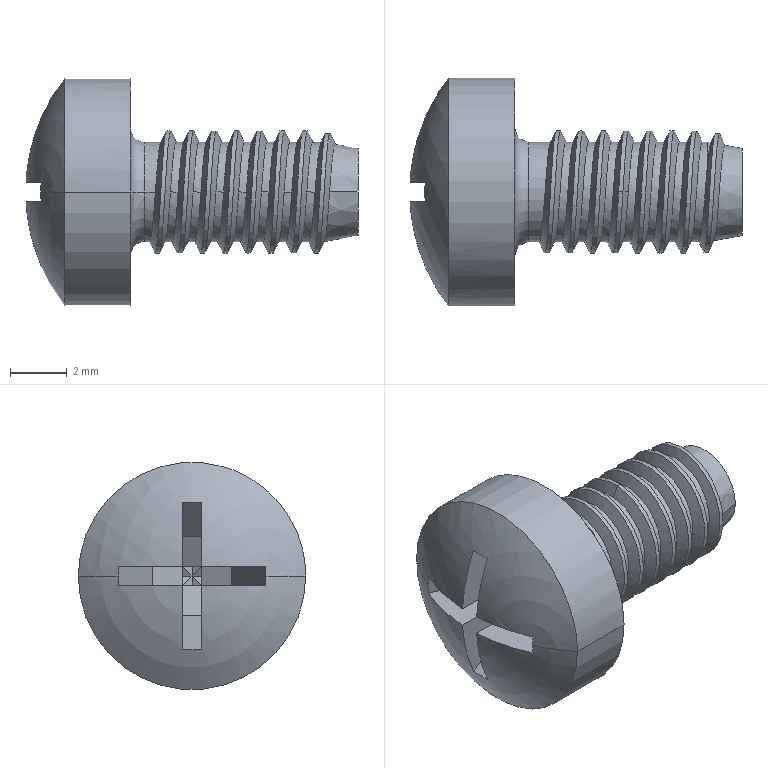Part | STEP file | RJWD-DY-0102_X2_5DE667DC95E8_14 | 1 solid | 64 faces | box 11.681 x 8 x 8 mm | volume 225.554 mm3 | plane 32 | cylinder 17 | spline 8 | cone 2 | torus 2 | sphere 2 | other 1 | commonest cylinder face diameters 3.5 x15 8 x2